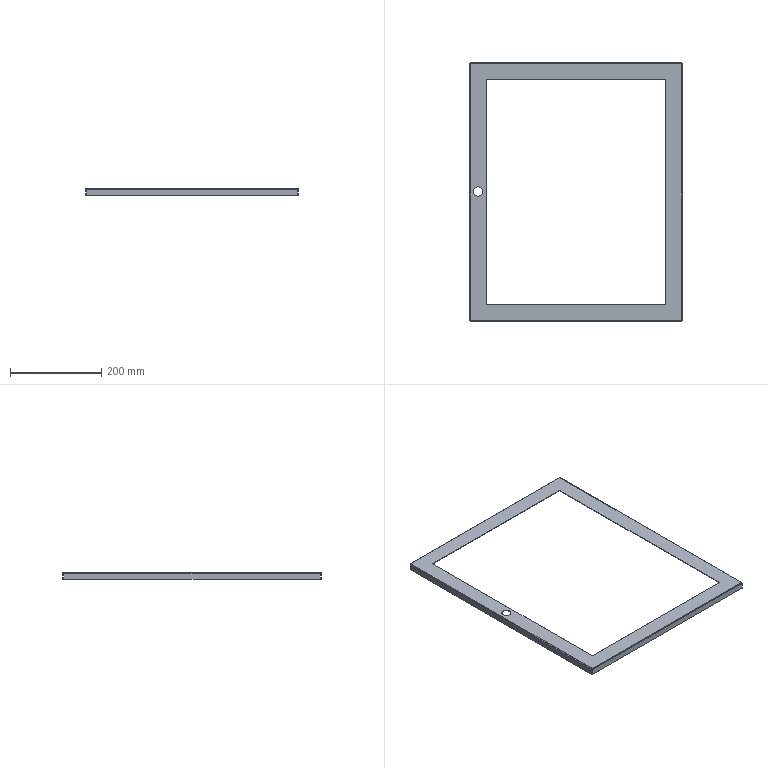Part | STEP file | x77-05402 | 1 solid | 44 faces | box 465.4 x 565.4 x 15 mm | volume 115350 mm3 | plane 26 | cylinder 10 | spline 8 | commonest cylinder face diameters 1.473 x4 3.873 x4 20 x2